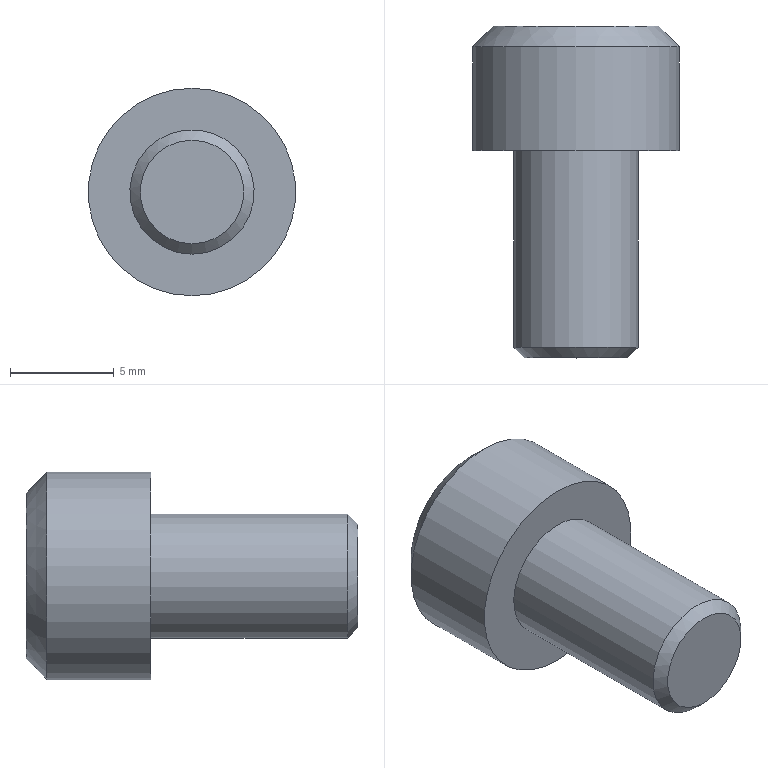Part | NX | features solid 2 | 1 solid | 14 faces | box 10 x 16 x 10 mm | volume 612.389 mm3 | plane 10 | cylinder 2 | cone 2 | commonest cylinder face diameters 6 x1 10 x1
STEP:
#1=CARTESIAN_POINT('',(0.,715.,-138.));
#2=VERTEX_POINT('',#1);
#3=CARTESIAN_POINT('',(0.,715.,-143.));
#4=DIRECTION('',(0.,1.,0.));
#5=DIRECTION('',(0.,0.,1.));
#6=AXIS2_PLACEMENT_3D('',#3,#4,#5);
#7=CIRCLE('',#6,5.);
#8=EDGE_CURVE('',#2,#2,#7,.F.);
#9=ORIENTED_EDGE('',*,*,#8,.T.);
#10=EDGE_LOOP('',(#9));
#11=FACE_BOUND('',#10,.T.);
#12=CARTESIAN_POINT('',(0.,710.,-138.));
#13=VERTEX_POINT('',#12);
#14=CARTESIAN_POINT('',(0.,710.,-143.));
#15=DIRECTION('',(0.,1.,0.));
#16=DIRECTION('',(0.,0.,1.));
#17=AXIS2_PLACEMENT_3D('',#14,#15,#16);
#18=CIRCLE('',#17,5.);
#19=EDGE_CURVE('',#13,#13,#18,.T.);
#20=ORIENTED_EDGE('',*,*,#19,.T.);
#21=EDGE_LOOP('',(#20));
#22=FACE_BOUND('',#21,.T.);
#23=CARTESIAN_POINT('',(0.,710.,-143.));
#24=DIRECTION('',(0.,1.,0.));
#25=DIRECTION('',(0.,0.,1.));
#26=AXIS2_PLACEMENT_3D('',#23,#24,#25);
#27=CYLINDRICAL_SURFACE('',#26,5.);
#28=ADVANCED_FACE('',(#11,#22),#27,.T.);
#29=CARTESIAN_POINT('',(0.,710.,-146.));
#30=VERTEX_POINT('',#29);
#31=CARTESIAN_POINT('',(0.,710.,-143.));
#32=DIRECTION('',(0.,-1.,0.));
#33=DIRECTION('',(0.,0.,-1.));
#34=AXIS2_PLACEMENT_3D('',#31,#32,#33);
#35=CIRCLE('',#34,3.);
#36=EDGE_CURVE('',#30,#30,#35,.T.);
#37=ORIENTED_EDGE('',*,*,#36,.F.);
#38=EDGE_LOOP('',(#37));
#39=FACE_BOUND('',#38,.T.);
#40=ORIENTED_EDGE('',*,*,#19,.F.);
#41=EDGE_LOOP('',(#40));
#42=FACE_BOUND('',#41,.T.);
#43=CARTESIAN_POINT('',(0.,710.,-143.));
#44=DIRECTION('',(0.,1.,0.));
#45=DIRECTION('',(0.,0.,1.));
#46=AXIS2_PLACEMENT_3D('',#43,#44,#45);
#47=PLANE('',#46);
#48=ADVANCED_FACE('',(#39,#42),#47,.F.);
#49=CARTESIAN_POINT('',(0.,716.,-139.));
#50=VERTEX_POINT('',#49);
#51=CARTESIAN_POINT('',(0.,716.,-143.));
#52=DIRECTION('',(0.,1.,0.));
#53=DIRECTION('',(0.,0.,1.));
#54=AXIS2_PLACEMENT_3D('',#51,#52,#53);
#55=CIRCLE('',#54,4.);
#56=EDGE_CURVE('',#50,#50,#55,.T.);
#57=ORIENTED_EDGE('',*,*,#56,.T.);
#58=EDGE_LOOP('',(#57));
#59=FACE_BOUND('',#58,.T.);
#60=CARTESIAN_POINT('',(3.,716.,-144.732));
#61=VERTEX_POINT('',#60);
#62=CARTESIAN_POINT('',(0.,716.,-146.464));
#63=VERTEX_POINT('',#62);
#64=CARTESIAN_POINT('',(3.,716.,-144.732));
#65=DIRECTION('',(-0.866,0.,-0.5));
#66=VECTOR('',#65,1000.);
#67=LINE('',#64,#66);
#68=EDGE_CURVE('',#61,#63,#67,.T.);
#69=ORIENTED_EDGE('',*,*,#68,.F.);
#70=CARTESIAN_POINT('',(3.,716.,-141.268));
#71=VERTEX_POINT('',#70);
#72=CARTESIAN_POINT('',(3.,716.,-141.268));
#73=DIRECTION('',(0.,0.,-1.));
#74=VECTOR('',#73,1000.);
#75=LINE('',#72,#74);
#76=EDGE_CURVE('',#71,#61,#75,.T.);
#77=ORIENTED_EDGE('',*,*,#76,.F.);
#78=CARTESIAN_POINT('',(0.,716.,-139.536));
#79=VERTEX_POINT('',#78);
#80=CARTESIAN_POINT('',(0.,716.,-139.536));
#81=DIRECTION('',(0.866,0.,-0.5));
#82=VECTOR('',#81,1000.);
#83=LINE('',#80,#82);
#84=EDGE_CURVE('',#79,#71,#83,.T.);
#85=ORIENTED_EDGE('',*,*,#84,.F.);
#86=CARTESIAN_POINT('',(-3.,716.,-141.268));
#87=VERTEX_POINT('',#86);
#88=CARTESIAN_POINT('',(-3.,716.,-141.268));
#89=DIRECTION('',(0.866,0.,0.5));
#90=VECTOR('',#89,1000.);
#91=LINE('',#88,#90);
#92=EDGE_CURVE('',#87,#79,#91,.T.);
#93=ORIENTED_EDGE('',*,*,#92,.F.);
#94=CARTESIAN_POINT('',(-3.,716.,-144.732));
#95=VERTEX_POINT('',#94);
#96=CARTESIAN_POINT('',(-3.,716.,-144.732));
#97=DIRECTION('',(0.,0.,1.));
#98=VECTOR('',#97,1000.);
#99=LINE('',#96,#98);
#100=EDGE_CURVE('',#95,#87,#99,.T.);
#101=ORIENTED_EDGE('',*,*,#100,.F.);
#102=CARTESIAN_POINT('',(0.,716.,-146.464));
#103=DIRECTION('',(-0.866,0.,0.5));
#104=VECTOR('',#103,1000.);
#105=LINE('',#102,#104);
#106=EDGE_CURVE('',#63,#95,#105,.T.);
#107=ORIENTED_EDGE('',*,*,#106,.F.);
#108=EDGE_LOOP('',(#69,#77,#85,#93,#101,#107));
#109=FACE_BOUND('',#108,.T.);
#110=CARTESIAN_POINT('',(0.,716.,-143.));
#111=DIRECTION('',(0.,1.,0.));
#112=DIRECTION('',(0.,0.,1.));
#113=AXIS2_PLACEMENT_3D('',#110,#111,#112);
#114=PLANE('',#113);
#115=ADVANCED_FACE('',(#59,#109),#114,.T.);
#116=CARTESIAN_POINT('',(0.,700.,-145.5));
#117=VERTEX_POINT('',#116);
#118=CARTESIAN_POINT('',(0.,700.,-143.));
#119=DIRECTION('',(0.,-1.,0.));
#120=DIRECTION('',(0.,0.,-1.));
#121=AXIS2_PLACEMENT_3D('',#118,#119,#120);
#122=CIRCLE('',#121,2.5);
#123=EDGE_CURVE('',#117,#117,#122,.T.);
#124=ORIENTED_EDGE('',*,*,#123,.T.);
#125=EDGE_LOOP('',(#124));
#126=FACE_BOUND('',#125,.T.);
#127=CARTESIAN_POINT('',(0.,700.,-143.));
#128=DIRECTION('',(0.,-1.,0.));
#129=DIRECTION('',(0.,0.,-1.));
#130=AXIS2_PLACEMENT_3D('',#127,#128,#129);
#131=PLANE('',#130);
#132=ADVANCED_FACE('',(#126),#131,.T.);
#133=CARTESIAN_POINT('',(0.,700.5,-146.));
#134=VERTEX_POINT('',#133);
#135=CARTESIAN_POINT('',(0.,700.5,-143.));
#136=DIRECTION('',(0.,-1.,0.));
#137=DIRECTION('',(0.,0.,-1.));
#138=AXIS2_PLACEMENT_3D('',#135,#136,#137);
#139=CIRCLE('',#138,3.);
#140=EDGE_CURVE('',#134,#134,#139,.F.);
#141=ORIENTED_EDGE('',*,*,#140,.T.);
#142=EDGE_LOOP('',(#141));
#143=FACE_BOUND('',#142,.T.);
#144=ORIENTED_EDGE('',*,*,#36,.T.);
#145=EDGE_LOOP('',(#144));
#146=FACE_BOUND('',#145,.T.);
#147=CARTESIAN_POINT('',(0.,710.,-143.));
#148=DIRECTION('',(0.,-1.,0.));
#149=DIRECTION('',(0.,0.,-1.));
#150=AXIS2_PLACEMENT_3D('',#147,#148,#149);
#151=CYLINDRICAL_SURFACE('',#150,3.);
#152=ADVANCED_FACE('',(#143,#146),#151,.T.);
#153=ORIENTED_EDGE('',*,*,#68,.T.);
#154=CARTESIAN_POINT('',(0.,712.,-146.464));
#155=VERTEX_POINT('',#154);
#156=CARTESIAN_POINT('',(0.,712.,-146.464));
#157=DIRECTION('',(0.,1.,0.));
#158=VECTOR('',#157,1000.);
#159=LINE('',#156,#158);
#160=EDGE_CURVE('',#155,#63,#159,.T.);
#161=ORIENTED_EDGE('',*,*,#160,.F.);
#162=CARTESIAN_POINT('',(3.,712.,-144.732));
#163=VERTEX_POINT('',#162);
#164=CARTESIAN_POINT('',(3.,712.,-144.732));
#165=DIRECTION('',(-0.866,0.,-0.5));
#166=VECTOR('',#165,1000.);
#167=LINE('',#164,#166);
#168=EDGE_CURVE('',#163,#155,#167,.T.);
#169=ORIENTED_EDGE('',*,*,#168,.F.);
#170=CARTESIAN_POINT('',(3.,712.,-144.732));
#171=DIRECTION('',(0.,1.,0.));
#172=VECTOR('',#171,1000.);
#173=LINE('',#170,#172);
#174=EDGE_CURVE('',#163,#61,#173,.T.);
#175=ORIENTED_EDGE('',*,*,#174,.T.);
#176=EDGE_LOOP('',(#153,#161,#169,#175));
#177=FACE_BOUND('',#176,.T.);
#178=CARTESIAN_POINT('',(3.,712.,-144.732));
#179=DIRECTION('',(0.5,0.,-0.866));
#180=DIRECTION('',(-0.866,0.,-0.5));
#181=AXIS2_PLACEMENT_3D('',#178,#179,#180);
#182=PLANE('',#181);
#183=ADVANCED_FACE('',(#177),#182,.F.);
#184=ORIENTED_EDGE('',*,*,#106,.T.);
#185=CARTESIAN_POINT('',(-3.,712.,-144.732));
#186=VERTEX_POINT('',#185);
#187=CARTESIAN_POINT('',(-3.,712.,-144.732));
#188=DIRECTION('',(0.,1.,0.));
#189=VECTOR('',#188,1000.);
#190=LINE('',#187,#189);
#191=EDGE_CURVE('',#186,#95,#190,.T.);
#192=ORIENTED_EDGE('',*,*,#191,.F.);
#193=CARTESIAN_POINT('',(0.,712.,-146.464));
#194=DIRECTION('',(-0.866,0.,0.5));
#195=VECTOR('',#194,1000.);
#196=LINE('',#193,#195);
#197=EDGE_CURVE('',#155,#186,#196,.T.);
#198=ORIENTED_EDGE('',*,*,#197,.F.);
#199=ORIENTED_EDGE('',*,*,#160,.T.);
#200=EDGE_LOOP('',(#184,#192,#198,#199));
#201=FACE_BOUND('',#200,.T.);
#202=CARTESIAN_POINT('',(0.,712.,-146.464));
#203=DIRECTION('',(-0.5,0.,-0.866));
#204=DIRECTION('',(-0.866,0.,0.5));
#205=AXIS2_PLACEMENT_3D('',#202,#203,#204);
#206=PLANE('',#205);
#207=ADVANCED_FACE('',(#201),#206,.F.);
#208=ORIENTED_EDGE('',*,*,#100,.T.);
#209=CARTESIAN_POINT('',(-3.,712.,-141.268));
#210=VERTEX_POINT('',#209);
#211=CARTESIAN_POINT('',(-3.,712.,-141.268));
#212=DIRECTION('',(0.,1.,0.));
#213=VECTOR('',#212,1000.);
#214=LINE('',#211,#213);
#215=EDGE_CURVE('',#210,#87,#214,.T.);
#216=ORIENTED_EDGE('',*,*,#215,.F.);
#217=CARTESIAN_POINT('',(-3.,712.,-144.732));
#218=DIRECTION('',(0.,0.,1.));
#219=VECTOR('',#218,1000.);
#220=LINE('',#217,#219);
#221=EDGE_CURVE('',#186,#210,#220,.T.);
#222=ORIENTED_EDGE('',*,*,#221,.F.);
#223=ORIENTED_EDGE('',*,*,#191,.T.);
#224=EDGE_LOOP('',(#208,#216,#222,#223));
#225=FACE_BOUND('',#224,.T.);
#226=CARTESIAN_POINT('',(-3.,712.,-144.732));
#227=DIRECTION('',(-1.,0.,0.));
#228=DIRECTION('',(0.,-1.,0.));
#229=AXIS2_PLACEMENT_3D('',#226,#227,#228);
#230=PLANE('',#229);
#231=ADVANCED_FACE('',(#225),#230,.F.);
#232=ORIENTED_EDGE('',*,*,#92,.T.);
#233=CARTESIAN_POINT('',(0.,712.,-139.536));
#234=VERTEX_POINT('',#233);
#235=CARTESIAN_POINT('',(0.,712.,-139.536));
#236=DIRECTION('',(0.,1.,0.));
#237=VECTOR('',#236,1000.);
#238=LINE('',#235,#237);
#239=EDGE_CURVE('',#234,#79,#238,.T.);
#240=ORIENTED_EDGE('',*,*,#239,.F.);
#241=CARTESIAN_POINT('',(-3.,712.,-141.268));
#242=DIRECTION('',(0.866,0.,0.5));
#243=VECTOR('',#242,1000.);
#244=LINE('',#241,#243);
#245=EDGE_CURVE('',#210,#234,#244,.T.);
#246=ORIENTED_EDGE('',*,*,#245,.F.);
#247=ORIENTED_EDGE('',*,*,#215,.T.);
#248=EDGE_LOOP('',(#232,#240,#246,#247));
#249=FACE_BOUND('',#248,.T.);
#250=CARTESIAN_POINT('',(-3.,712.,-141.268));
#251=DIRECTION('',(-0.5,0.,0.866));
#252=DIRECTION('',(0.866,0.,0.5));
#253=AXIS2_PLACEMENT_3D('',#250,#251,#252);
#254=PLANE('',#253);
#255=ADVANCED_FACE('',(#249),#254,.F.);
#256=ORIENTED_EDGE('',*,*,#84,.T.);
#257=CARTESIAN_POINT('',(3.,712.,-141.268));
#258=VERTEX_POINT('',#257);
#259=CARTESIAN_POINT('',(3.,712.,-141.268));
#260=DIRECTION('',(0.,1.,0.));
#261=VECTOR('',#260,1000.);
#262=LINE('',#259,#261);
#263=EDGE_CURVE('',#258,#71,#262,.T.);
#264=ORIENTED_EDGE('',*,*,#263,.F.);
#265=CARTESIAN_POINT('',(0.,712.,-139.536));
#266=DIRECTION('',(0.866,0.,-0.5));
#267=VECTOR('',#266,1000.);
#268=LINE('',#265,#267);
#269=EDGE_CURVE('',#234,#258,#268,.T.);
#270=ORIENTED_EDGE('',*,*,#269,.F.);
#271=ORIENTED_EDGE('',*,*,#239,.T.);
#272=EDGE_LOOP('',(#256,#264,#270,#271));
#273=FACE_BOUND('',#272,.T.);
#274=CARTESIAN_POINT('',(0.,712.,-139.536));
#275=DIRECTION('',(0.5,0.,0.866));
#276=DIRECTION('',(0.866,0.,-0.5));
#277=AXIS2_PLACEMENT_3D('',#274,#275,#276);
#278=PLANE('',#277);
#279=ADVANCED_FACE('',(#273),#278,.F.);
#280=ORIENTED_EDGE('',*,*,#76,.T.);
#281=ORIENTED_EDGE('',*,*,#174,.F.);
#282=CARTESIAN_POINT('',(3.,712.,-141.268));
#283=DIRECTION('',(0.,0.,-1.));
#284=VECTOR('',#283,1000.);
#285=LINE('',#282,#284);
#286=EDGE_CURVE('',#258,#163,#285,.T.);
#287=ORIENTED_EDGE('',*,*,#286,.F.);
#288=ORIENTED_EDGE('',*,*,#263,.T.);
#289=EDGE_LOOP('',(#280,#281,#287,#288));
#290=FACE_BOUND('',#289,.T.);
#291=CARTESIAN_POINT('',(3.,712.,-141.268));
#292=DIRECTION('',(1.,0.,0.));
#293=DIRECTION('',(0.,0.,-1.));
#294=AXIS2_PLACEMENT_3D('',#291,#292,#293);
#295=PLANE('',#294);
#296=ADVANCED_FACE('',(#290),#295,.F.);
#297=ORIENTED_EDGE('',*,*,#168,.T.);
#298=ORIENTED_EDGE('',*,*,#197,.T.);
#299=ORIENTED_EDGE('',*,*,#221,.T.);
#300=ORIENTED_EDGE('',*,*,#245,.T.);
#301=ORIENTED_EDGE('',*,*,#269,.T.);
#302=ORIENTED_EDGE('',*,*,#286,.T.);
#303=EDGE_LOOP('',(#297,#298,#299,#300,#301,#302));
#304=FACE_BOUND('',#303,.T.);
#305=CARTESIAN_POINT('',(0.,712.,-146.464));
#306=DIRECTION('',(0.,1.,0.));
#307=DIRECTION('',(0.,0.,1.));
#308=AXIS2_PLACEMENT_3D('',#305,#306,#307);
#309=PLANE('',#308);
#310=ADVANCED_FACE('',(#304),#309,.T.);
#311=ORIENTED_EDGE('',*,*,#8,.F.);
#312=EDGE_LOOP('',(#311));
#313=FACE_BOUND('',#312,.T.);
#314=ORIENTED_EDGE('',*,*,#56,.F.);
#315=EDGE_LOOP('',(#314));
#316=FACE_BOUND('',#315,.T.);
#317=CARTESIAN_POINT('',(0.,716.,-143.));
#318=DIRECTION('',(0.,-1.,0.));
#319=DIRECTION('',(0.,0.,-1.));
#320=AXIS2_PLACEMENT_3D('',#317,#318,#319);
#321=CONICAL_SURFACE('',#320,4.,0.7854);
#322=ADVANCED_FACE('',(#313,#316),#321,.T.);
#323=ORIENTED_EDGE('',*,*,#140,.F.);
#324=EDGE_LOOP('',(#323));
#325=FACE_BOUND('',#324,.T.);
#326=ORIENTED_EDGE('',*,*,#123,.F.);
#327=EDGE_LOOP('',(#326));
#328=FACE_BOUND('',#327,.T.);
#329=CARTESIAN_POINT('',(0.,700.,-143.));
#330=DIRECTION('',(0.,1.,0.));
#331=DIRECTION('',(0.,0.,1.));
#332=AXIS2_PLACEMENT_3D('',#329,#330,#331);
#333=CONICAL_SURFACE('',#332,2.5,0.7854);
#334=ADVANCED_FACE('',(#325,#328),#333,.T.);
#335=CLOSED_SHELL('',(#28,#48,#115,#132,#152,#183,#207,#231,#255,#279,#296,#310,#322,#334));
#336=MANIFOLD_SOLID_BREP('',#335);
#337=(LENGTH_UNIT()NAMED_UNIT(*)SI_UNIT(.MILLI.,.METRE.));
#338=UNCERTAINTY_MEASURE_WITH_UNIT(LENGTH_MEASURE(0.00001),#337,'','');
#339=(NAMED_UNIT(*)PLANE_ANGLE_UNIT()SI_UNIT($,.RADIAN.));
#340=(NAMED_UNIT(*)SI_UNIT($,.STERADIAN.)SOLID_ANGLE_UNIT());
#341=(GEOMETRIC_REPRESENTATION_CONTEXT(3)GLOBAL_UNCERTAINTY_ASSIGNED_CONTEXT((#338))GLOBAL_UNIT_ASSIGNED_CONTEXT((#337,#339,#340))REPRESENTATION_CONTEXT('',''));
#342=ADVANCED_BREP_SHAPE_REPRESENTATION('',(#336),#341);